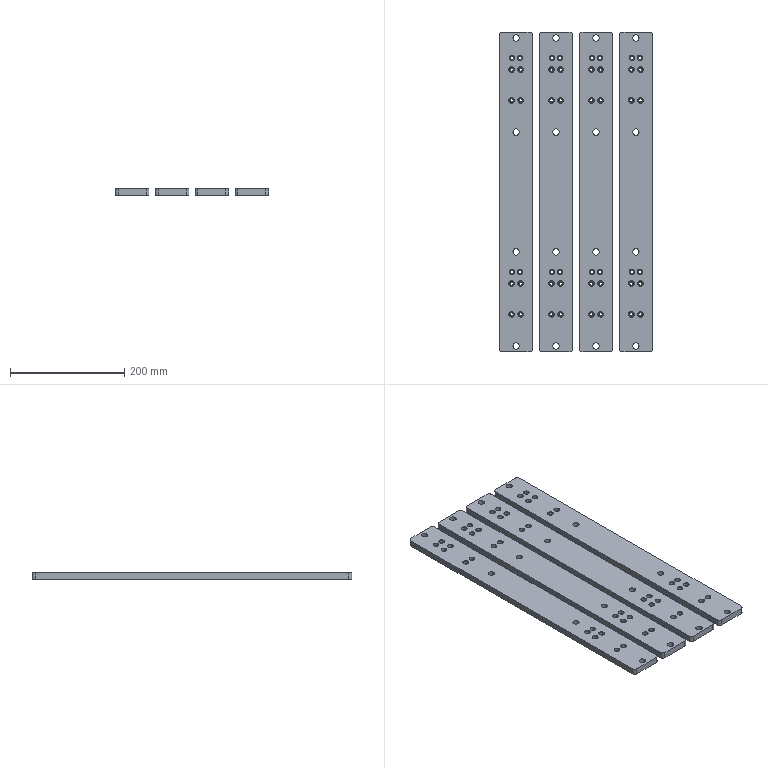Part | 4 solids | 352 faces | box 269 x 560 x 11 mm | volume 1386865 mm3 | cylinder 192 | plane 112 | cone 48 | commonest cylinder face diameters 5.5 x48 9 x48 3.9 x32 10.1 x32 10 x16 11 x16